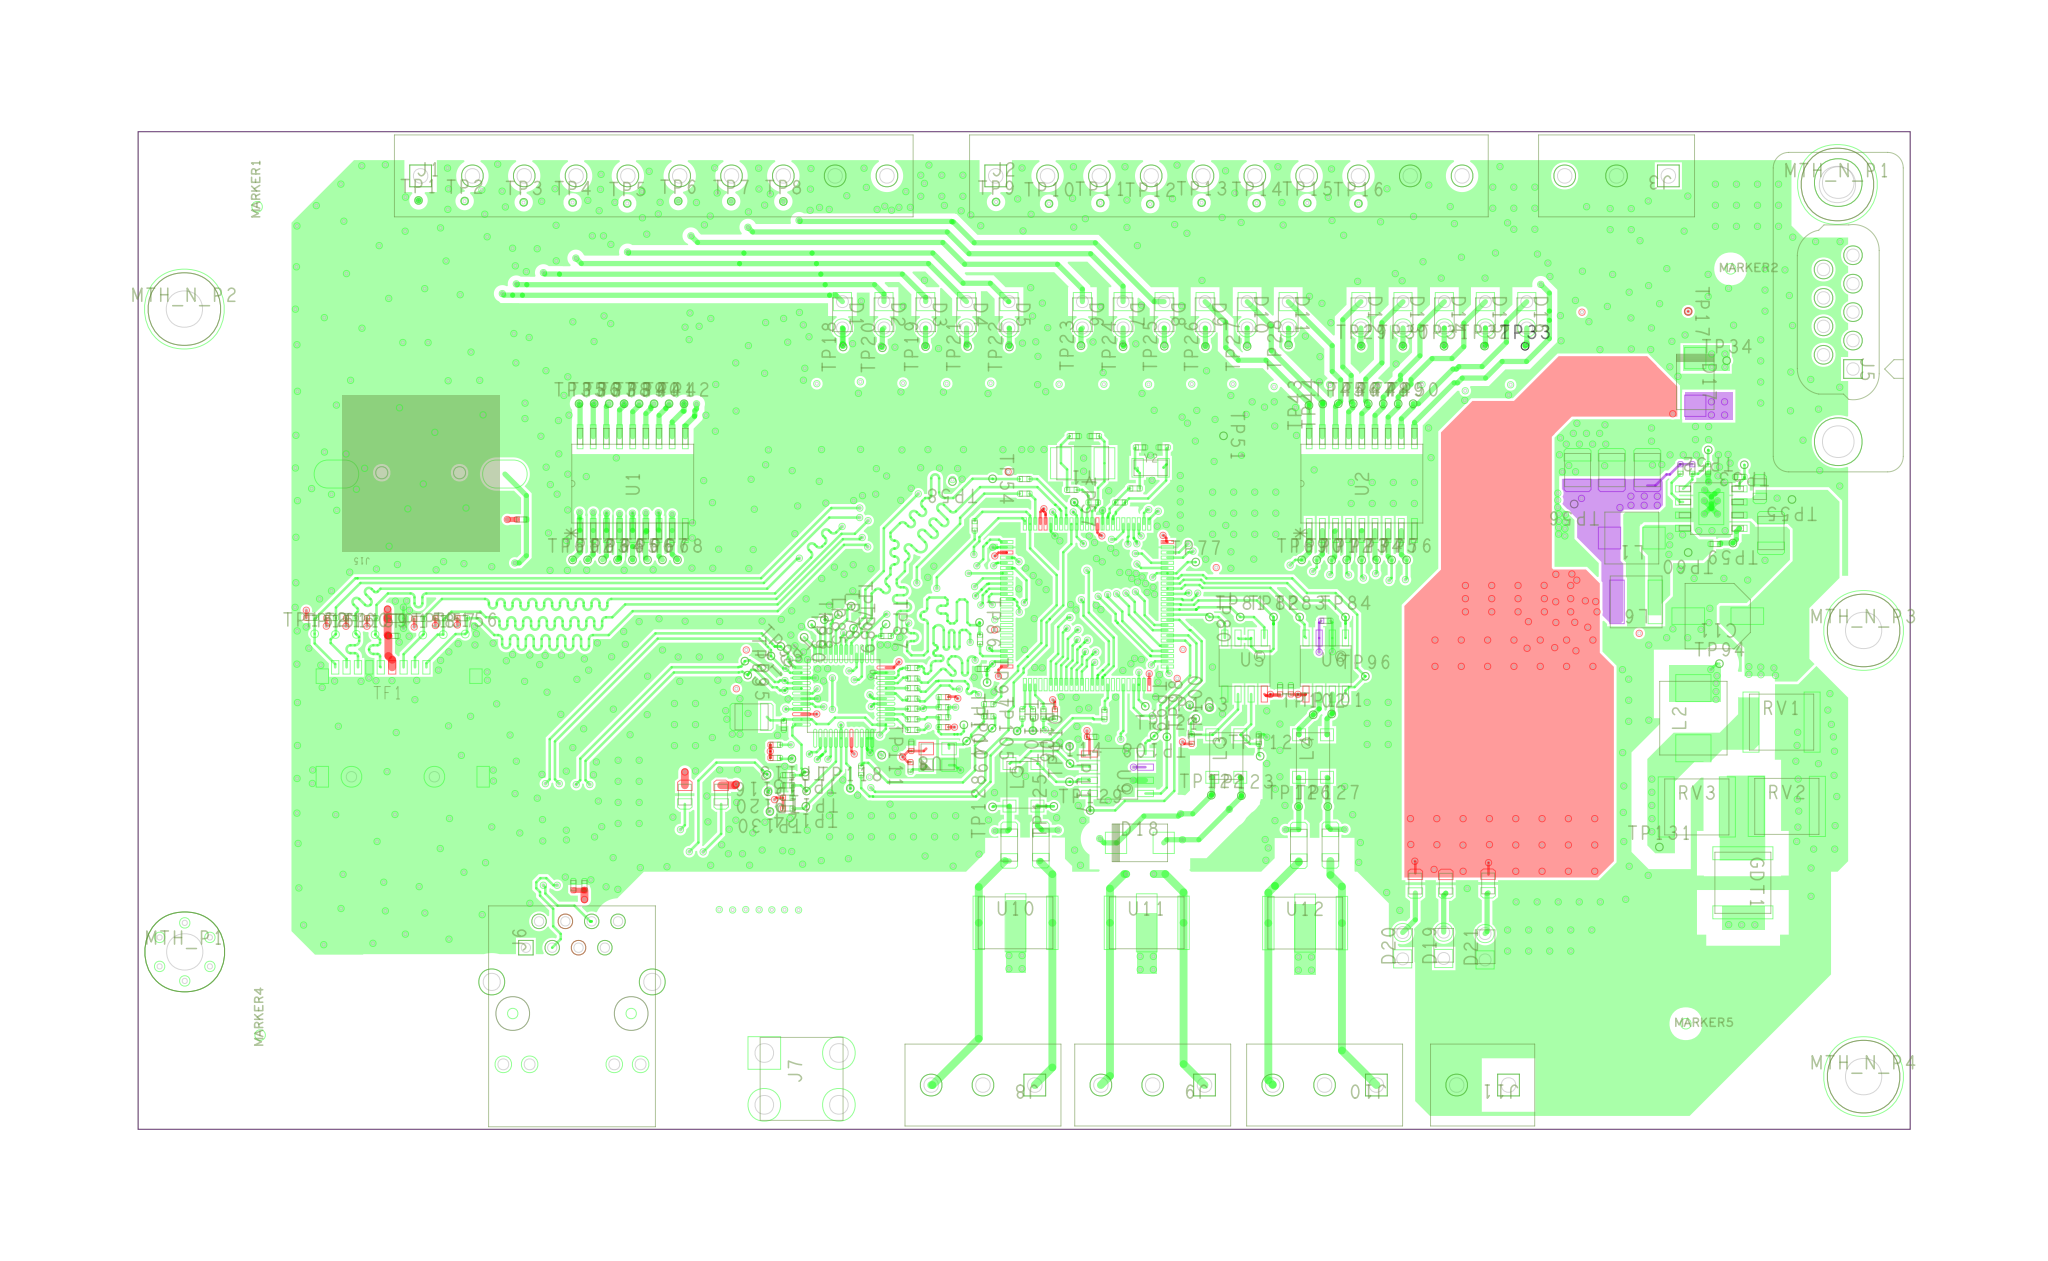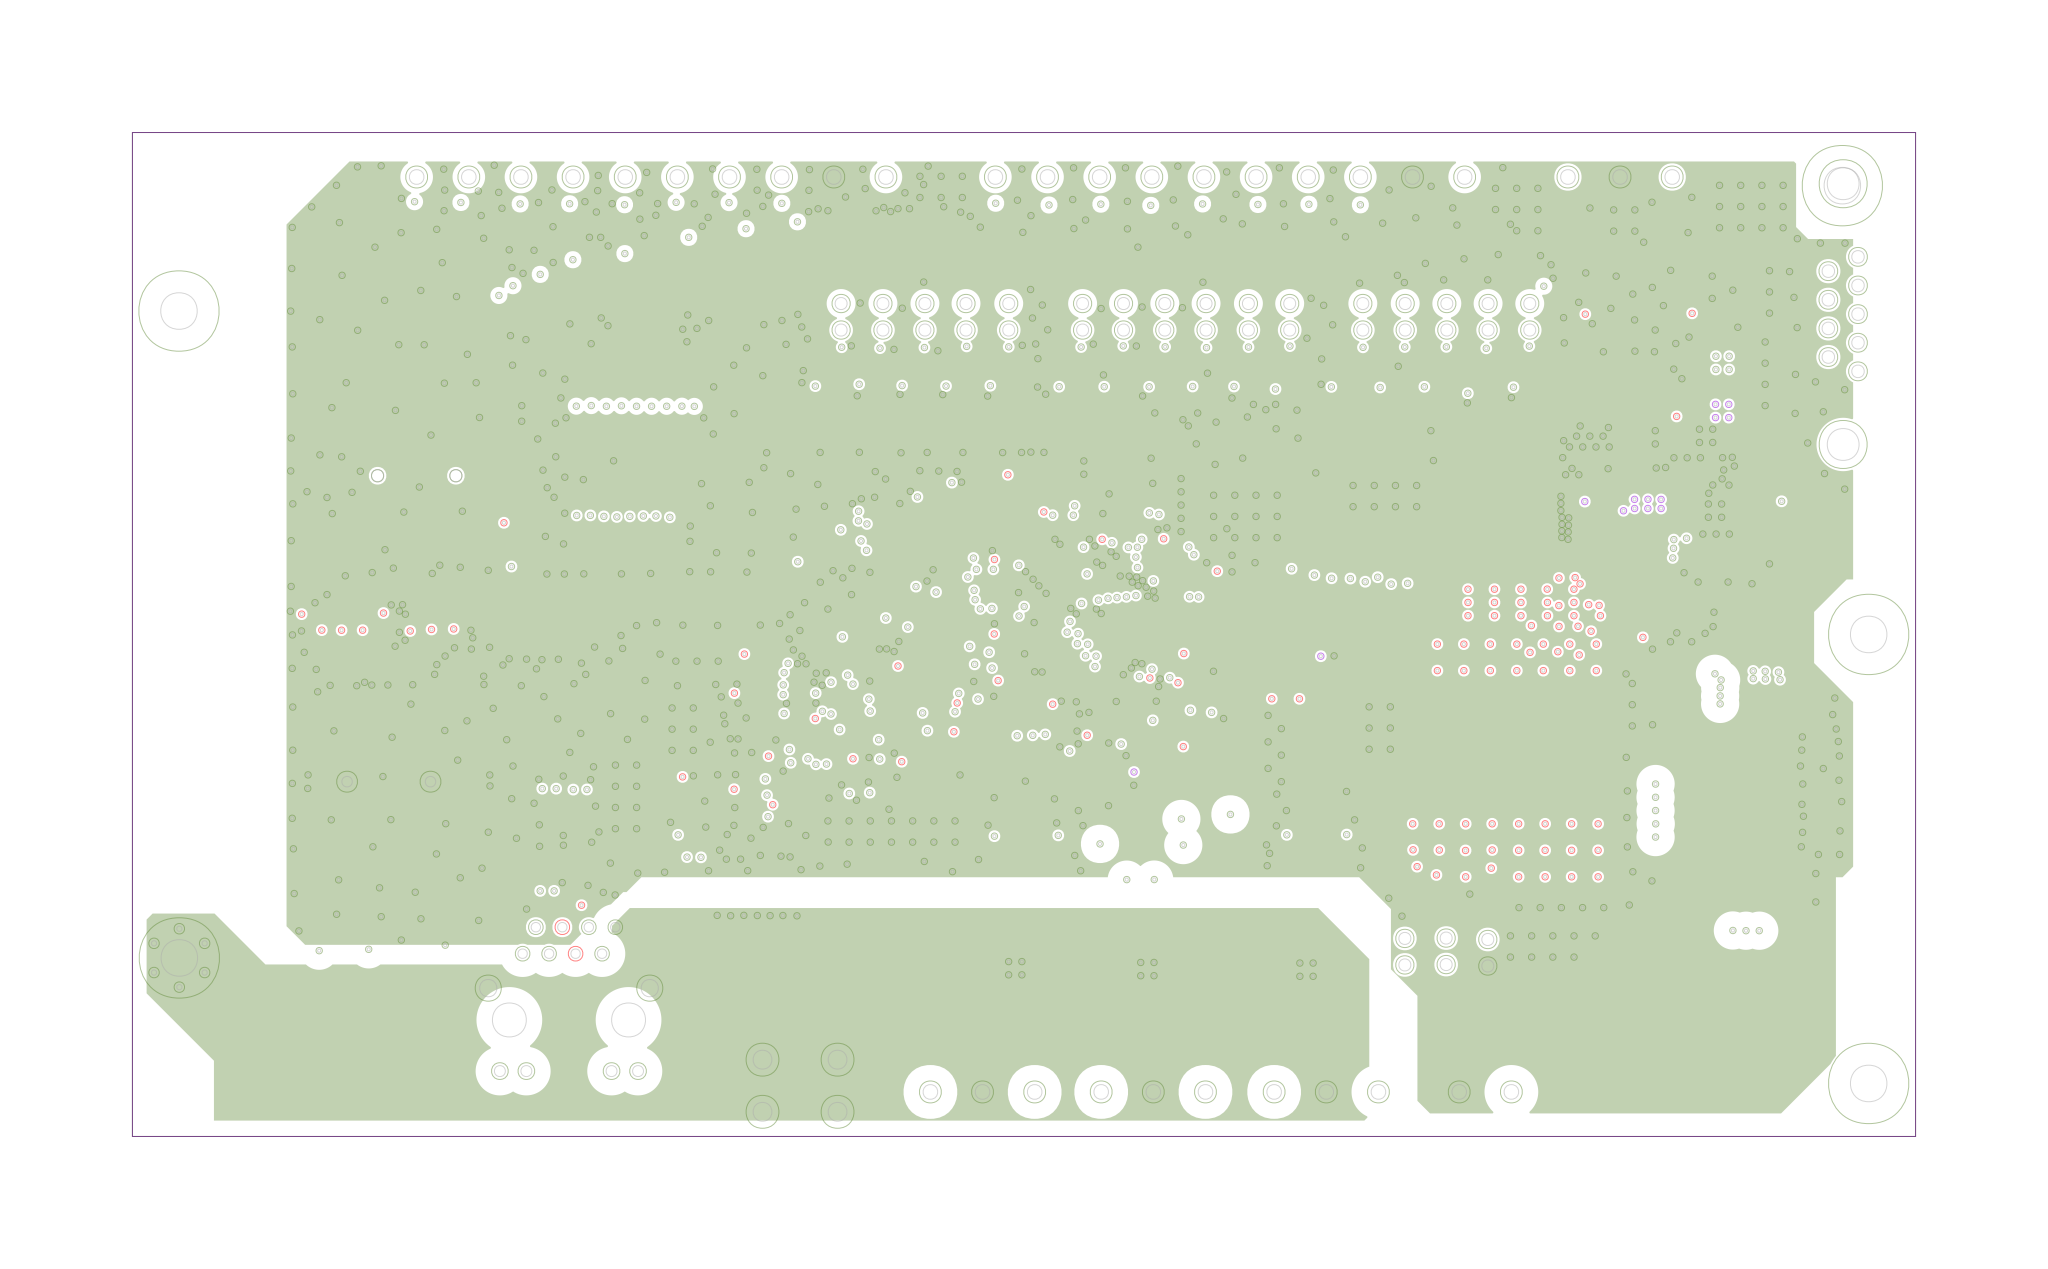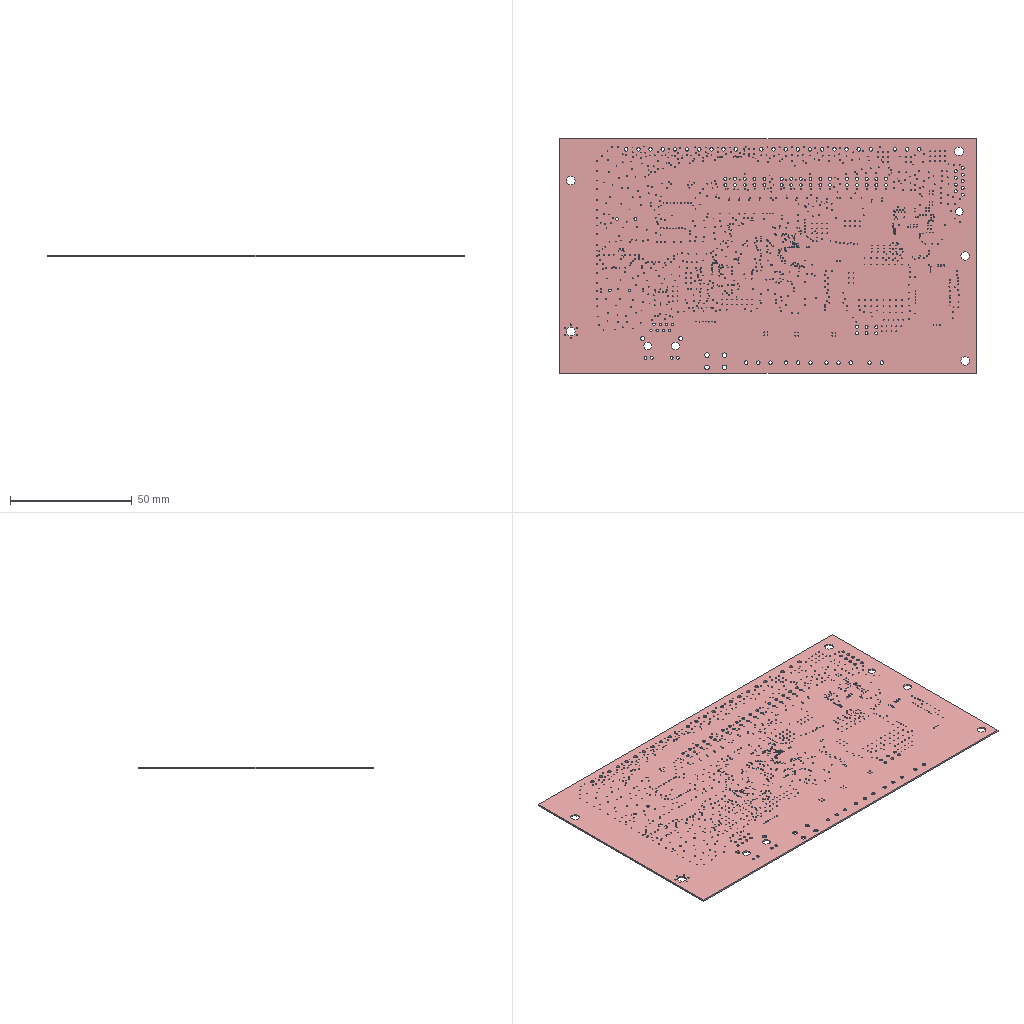Circuit board layout | Cadence Allegro | box 171 x 96.2 x 0.7 mm
Layer stack:
# Cadence Allegro layer stack of  (unit mm; from the constraint file cross-section; dielectric type: 0 not recorded (Allegro does not mark core vs prepreg), 3 surface material)
index,name,kind,layer,copper_thickness_mm,dielectric_type,dielectric_thickness_mm,dielectric_material,dielectric_constant
0,Top Surface,other,,,,,,
1,TOP,copper,TOP,0.0305,,,,
2,Dielectric1,dielectric,,,0,0.2032,FR-4,4.5
3,GND,copper,GND,0.0305,,,,
4,Dielectric2,dielectric,,,0,0.2032,FR-4,4.5
5,POWER,copper,POWER,0.0305,,,,
6,Dielectric3,dielectric,,,0,0.2032,FR-4,4.5
7,BOTTOM,copper,BOTTOM,0.0305,,,,
8,Bottom Surface,other,,,,,,
# drill layer pairs: low layer,high layer
drill_pair,TOP,BOTTOM
Part placement:
REFDES,COMP_VALUE,SYM_NAME,SYM_X,SYM_Y,SYM_ROTATE,SYM_MIRROR
C1,8PF,C0402,6855.4,7438.9,180.000,NO
C2,8PF,C0402,6931.2,7438.9,0.000,NO
C3,6PF,C0402,7106.7,7396.1,0.000,NO
C4,6PF,C0402,7192.7,7396.1,180.000,NO
C5,22uf,C1210,8767.0,7310.0,90.000,NO
C6,22uf,C1210,8897.0,7310.0,90.000,NO
C7,22uf,C1210,9032.0,7310.0,90.000,NO
C8,.22uf,C0805,9459.5,7237.7,90.000,NO
C9,4.7uf,C1210,9502.0,7071.0,270.000,NO
C10,.1uf,C0402,9290.0,7029.4,180.000,NO
C11,47uF,CAPAE630X770N,9299.6,6755.5,180.000,NO
C12,.1uf,C0402,7810.8,6737.8,180.000,NO
C13,.1uf,C0402,7637.0,6476.0,90.000,NO
C14,.1uf,C0402,7677.8,6476.0,90.000,NO
C15,10uf,C1210,5629.0,6373.0,180.000,NO
C16,.1uf,C0402,5751.5,6341.2,270.000,NO
C17,.1uf,C0402,6921.0,6297.0,0.000,NO
C18,.1uf,C0402,6236.0,6261.0,90.000,NO
C19,.1uf,C0402,5766.6,6112.8,180.000,NO
C20,.1uf,C0402,4952.1,5732.2,90.000,NO
C21,.1uf,C0402,4994.2,5731.7,90.000,NO
C22,10uf,C1210,8883.0,7307.0,0.000,YES
C23,.047uf,C0402,6454.5,7288.5,90.000,YES
C24,1uf,C0603,8901.0,7208.0,0.000,YES
C25,.1uf,C0402,6928.3,7163.6,90.000,YES
C26,.1uf,C0402,9106.6,7156.8,180.000,YES
C27,.1uf,C0402,6773.0,7207.4,270.000,YES
C28,1uf,C0603,6725.9,7224.5,270.000,YES
C29,.1uf,C0402,8652.4,7044.0,270.000,YES
C30,10uf,C1210,8564.0,7046.0,270.000,YES
C31,22uf,C1210,8415.1,7046.0,270.000,YES
C32,.1uf,C0402,7152.0,7037.0,0.000,YES
C33,.1uf,C0402,6969.6,7107.0,270.000,YES
C34,.1uf,C0402,6586.8,6986.9,270.000,YES
C35,.1uf,C0402,6867.2,7062.2,180.000,YES
C36,.047uf,C0402,6594.5,6916.1,180.000,YES
C37,.047uf,C0402,6594.8,6835.9,180.000,YES
C38,.047uf,C0402,6690.6,6722.7,180.000,YES
C39,10uf,C1210,6119.0,6632.0,270.000,YES
C40,2.2uf,C0603,6606.0,6627.0,180.000,YES
C41,.1uf,C0402,6220.5,6612.0,270.000,YES
C42,.1uf,C0402,5609.0,6587.0,90.000,YES
C43,.1uf,C0402,6607.0,6577.0,180.000,YES
C44,10uf,C1210,6662.0,6492.0,180.000,YES
C45,.1uf,C0402,7127.0,6467.0,90.000,YES
C46,.1uf,C0402,5849.0,6462.0,90.000,YES
C47,.1uf,C0402,5609.0,6462.0,90.000,YES
C48,2.2uf,C0603,7078.0,6459.0,90.000,YES
C49,.047uf,C0805,9617.0,6398.0,90.000,YES
C50,.1uf,C0402,5834.0,6357.0,0.000,YES
C51,.1uf,C0402,6129.0,6272.0,180.000,YES
C52,.1uf,C0402,6045.0,6272.0,180.000,YES
C53,.1uf,C0402,7135.0,6181.0,0.000,YES
C54,4700pf,C0603,6690.0,6178.0,0.000,YES
C55,4700pf,C0603,7790.0,6177.0,0.000,YES
C56,100PF,C0603,6568.0,5864.0,90.000,YES
C57,100PF,C0603,7878.4,5863.4,90.000,YES
C58,100PF,C0603,7656.7,5863.4,90.000,YES
C59,100PF,C0603,6781.0,5863.0,90.000,YES
C60,10nF,C1206,5675.7,5756.3,90.000,YES
C61,47nf,C1210,5549.0,5754.3,90.000,YES
C62,.1uf,C0402,4266.9,6680.5,0.000,NO
C63,2.2uf,C0603,4276.5,6747.0,0.000,NO
D1,LED,LEDRR254,5974.2,7899.6,270.000,NO
D2,LED,LEDRR254,6132.1,7899.6,270.000,NO
D3,LED,LEDRR254,6290.6,7899.6,270.000,NO
D4,LED,LEDRR254,6445.7,7899.6,270.000,NO
D5,LED,LEDRR254,6607.0,7899.6,270.000,NO
D6,LED,LEDRR254,6885.9,7899.6,270.000,NO
D7,LED,LEDRR254,7040.4,7899.6,270.000,NO
D8,LED,LEDRR254,7196.2,7899.6,270.000,NO
D9,LED,LEDRR254,7352.0,7899.6,270.000,NO
D10,LED,LEDRR254,7511.9,7899.6,270.000,NO
D11,LED,LEDRR254,7667.8,7899.6,270.000,NO
D12,LED,LEDRR254,7943.9,7899.6,270.000,NO
D13,LED,LEDRR254,8103.8,7899.6,270.000,NO
D14,LED,LEDRR254,8261.0,7899.6,270.000,NO
D15,LED,LEDRR254,8416.8,7899.6,270.000,NO
D16,LED,LEDRR254,8574.1,7899.6,270.000,NO
D17,3A,SMB,9214.2,7644.7,270.000,NO
D18,SMBJ10CA,SMB,7104.2,5894.6,0.000,NO
D19,LED,LEDRR254,8258.5,5505.6,90.000,NO
D20,LED,LEDRR254,8102.6,5504.2,90.000,NO
D21,LED,LEDRR254,8415.7,5500.2,90.000,NO
D22,BAV99,SOT-23,9196.6,8009.0,270.000,YES
D23,BAV99,SOT-23,8841.3,8009.0,270.000,YES
D24,SS26FL,SMA,9046.0,7449.0,180.000,YES
D25,SS26FL,SMA,9262.0,7013.0,180.000,YES
D26,TPSMC27CA,SMC,9187.0,6388.0,270.000,YES
D27,3A,SMB,9482.0,6353.0,90.000,YES
D28,SMBJ10CA,SMB,7504.4,6119.4,90.000,YES
D29,SMBJ10CA,SMB,7322.4,6119.4,90.000,YES
D30,UFS08A2.8L04,SOIC127P600X175-8N,4928.2,5939.4,270.000,YES
D31,SM24CANA-04HTG,SOT23,6674.0,5853.0,180.000,YES
D32,SM24CANA-04HTG,SOT23,7768.0,5852.0,180.000,YES
D33,BAV99,SOT-23,4812.0,7570.5,180.000,YES
D34,1N4148WS,SOD-323,5949.9,7724.9,180.000,YES
D35,1N4148WS,SOD-323,6117.1,7726.5,180.000,YES
D36,1N4148WS,SOD-323,6281.5,7725.8,180.000,YES
D37,1N4148WS,SOD-323,6448.9,7725.2,180.000,YES
D38,1N4148WS,SOD-323,6613.1,7725.7,180.000,YES
D39,1N4148WS,SOD-323,6873.4,7724.2,180.000,YES
D40,1N4148WS,SOD-323,7042.0,7725.1,180.000,YES
D41,1N4148WS,SOD-323,7208.3,7725.0,180.000,YES
D42,1N4148WS,SOD-323,7373.0,7725.5,180.000,YES
D43,1N4148WS,SOD-323,7536.2,7726.1,180.000,YES
D44,1N4148WS,SOD-323,7698.0,7726.5,180.000,YES
D45,1N4148WS,SOD-323,7914.2,7724.4,180.000,YES
D46,1N4148WS,SOD-323,8079.4,7724.5,180.000,YES
D47,1N4148WS,SOD-323,8247.0,7725.0,180.000,YES
D48,1N4148WS,SOD-323,8416.1,7725.3,180.000,YES
D49,1N4148WS,SOD-323,8584.0,7725.4,180.000,YES
F1,10A,FUSE10A,9312.0,6068.0,0.000,YES
GDT1,5kA,GDT5KA2P,9395.0,5743.0,270.000,NO
J1,KF127-5.0-10P,PHONEX10P500_82,4371.7,8427.0,270.000,NO
J2,KF127-5.0-10P,PHONEX10P500_82,6556.6,8427.0,270.000,NO
J3,3,PHONEX3P500,9111.9,8427.0,90.000,NO
J5,DB9,DB_V_R-9,9813.4,7693.7,270.000,NO
J6,HY911105AE,RJ_RA-8,4771.7,5496.6,0.000,NO
J7,EARTH4P,EARTH4P_M3,5819.1,4998.4,0.000,NO
J8,KF127-5.0-3P,PHONEX3P500_82,6705.0,4975.0,90.000,NO
J9,KF127-5.0-3P,PHONEX3P500_82,7349.8,4975.1,90.000,NO
J10,KF127-5.0-3P,PHONEX3P500_82,8002.8,4975.1,90.000,NO
J11,KF127-5.0-2P,PHONEX2P500_82,8504.7,4975.1,90.000,NO
J13,TS5215A 250gf,TS5215A,4858.9,7099.9,90.000,YES
J15,BAT2,CR1220,4371.9,7299.9,180.000,NO
L1,6.8uH,SPM5030,8973.0,7052.0,180.000,NO
L2,22uH,SPM6530,9207.0,6368.0,90.000,NO
L3,51uH,CM320X450X150-4N,7432.5,6224.2,0.000,NO
L4,51uH,CM320X450X150-4N,7762.0,6224.2,0.000,NO
L5,51uH,CM320X450X150-4N,6662.0,6115.0,0.000,NO
L6,6.8uH,SNR5040,8989.7,6809.5,180.000,NO
MARKER1,30mil,FIDMS0,3750.6,8309.7,90.000,NO
MARKER2,30mil,FIDMS0,9348.4,8073.9,0.000,NO
MARKER3,30mil,FIDMS0,3982.6,5332.6,0.000,YES
MARKER4,30mil,FIDMS0,3762.1,5164.7,90.000,NO
MARKER5,30mil,FIDMS0,9178.4,5207.9,0.000,NO
MARKER6,30mil,FIDMS0,3802.6,8341.2,0.000,YES
MARKER7,30mil,FIDMS0,9431.0,8157.0,0.000,YES
MARKER8,30mil,FIDMS0,9179.1,5206.0,90.000,YES
MTH_N_P1,D3.5plated,MTGP770H350P,9754.3,8394.3,0.000,NO
MTH_N_P2,D3.5plated,MTGP770H350P,3474.3,7921.3,0.000,NO
MTH_N_P3,D3.5plated,MTGP770H350P,9853.7,6701.1,0.000,NO
MTH_N_P4,D3.5plated,MTGP770H350P,9853.7,5007.0,0.000,NO
MTH_P1,D3.5plated,MTGP770H350V6P,3475.7,5480.6,0.000,NO
R1,10k,R0402,9158.0,7314.0,90.000,NO
R2,68k,R0402,9203.0,7314.0,270.000,NO
R3,12k,R0402,9263.0,7314.0,270.000,NO
R4,16.9k,R0402,9383.0,7284.0,180.000,NO
R5,33R(NC),R0402,6666.7,7276.0,180.000,NO
R6,0R,R0402,7085.6,7240.2,0.000,NO
R7,0R,R0402,6846.0,7235.0,0.000,NO
R8,0R,R0402,6666.7,7220.5,180.000,NO
R9,1M,R0402,6927.0,7187.0,180.000,NO
R10,10M,R0402,7029.2,7187.0,0.000,NO
R11,0R,R0402,6476.6,7098.2,270.000,NO
R12,33R(NC),R0402,6140.0,6680.0,180.000,NO
R13,33R,R0402,6497.0,6667.0,90.000,NO
R14,33R(NC),R0402,6240.8,6558.5,180.000,NO
R15,0R(NC),R0402,6506.0,6555.0,180.000,NO
R16,33R(NC),R0402,6240.8,6518.5,180.000,NO
R17,33R,R0402,6240.8,6482.0,180.000,NO
R18,2.2k,R0402,6358.0,6447.9,180.000,NO
R19,33R,R0402,6240.8,6442.0,180.000,NO
R20,0R,R0402,6530.0,6421.0,180.000,NO
R21,0R,R0402,6358.0,6409.5,180.000,NO
R22,33R,R0402,6240.8,6403.9,180.000,NO
R23,33R,R0402,6658.0,6384.0,270.000,NO
R24,33R,R0402,6698.0,6384.0,270.000,NO
R25,0R(NC),R0402,6738.0,6384.0,90.000,NO
R26,10k(NC),R0402,6781.5,6384.0,270.000,NO
R27,33R,R0402,6969.5,6382.0,90.000,NO
R28,0R,R0402,6530.0,6375.0,0.000,NO
R29,0R,R0402,6358.0,6371.5,180.000,NO
R30,33R,R0402,6240.8,6363.9,180.000,NO
R31,2.2k,R0402,6358.0,6334.0,180.000,NO
R32,33R(NC),R0402,6240.9,6323.5,180.000,NO
R33,10k,R0402,7301.1,6288.6,90.000,NO
R34,10k,R0402,7556.1,6288.6,270.000,NO
R35,2.2k,R0402,5719.0,6267.0,180.000,NO
R36,2.2k,R0402,5719.0,6217.0,180.000,NO
R37,10k,R0402,6233.0,6183.0,90.000,NO
R38,0R(NC),R0402,6045.5,6169.5,90.000,NO
R39,4.87k,R0402,5766.6,6151.5,180.000,NO
R40,390R,R0805,5375.6,6077.7,90.000,NO
R41,390R,R0805,5513.5,6077.7,90.000,NO
R42,10k,R0402,5766.6,6066.0,0.000,NO
R43,1.5k,R0402,5766.6,6025.0,0.000,NO
R44,4.7R,R1206,6728.0,5887.0,270.000,NO
R45,4.7R,R1206,6608.0,5886.0,270.000,NO
R46,4.7R,R1206,7828.0,5886.0,270.000,NO
R47,4.7R,R1206,7708.0,5885.0,270.000,NO
R50,390R,R0805,8150.7,5739.7,90.000,NO
R51,1k,R0805,7941.5,8236.7,270.000,YES
R52,1k,R0805,7743.5,8239.0,270.000,YES
R53,1k,R0805,7550.4,8238.3,270.000,YES
R54,1k,R0805,7348.0,8240.6,270.000,YES
R55,1k,R0805,7154.5,8235.3,270.000,YES
R56,1k,R0805,6966.3,8238.7,270.000,YES
R57,1k,R0805,6764.0,8237.0,270.000,YES
R58,1k,R0805,6560.8,8235.8,270.000,YES
R59,1k,R0805,5751.4,8233.0,270.000,YES
R60,1k,R0805,5551.3,8233.9,270.000,YES
R61,1k,R0805,5354.2,8234.7,270.000,YES
R62,1k,R0805,5157.7,8226.2,270.000,YES
R63,1k,R0805,4961.5,8230.0,270.000,YES
R64,1k,R0805,4764.0,8231.2,270.000,YES
R65,1k,R0805,4550.9,8236.6,270.000,YES
R66,1k,R0805,4379.8,8236.6,270.000,YES
R67,4.7R,R1206,9175.1,8132.4,0.000,YES
R68,4.7R,R1206,8820.7,8132.4,0.000,YES
R101,2k,R0805,7209.5,7635.4,180.000,YES
R102,2k,R0805,7040.4,7635.9,180.000,YES
R103,2k,R0805,6869.5,7635.8,180.000,YES
R104,2k,R0805,6611.2,7638.1,180.000,YES
R105,2k,R0805,6442.4,7638.2,180.000,YES
R106,2k,R0805,6276.1,7640.0,180.000,YES
R107,2k,R0805,6114.5,7640.1,180.000,YES
R108,2k,R0805,5955.9,7638.5,180.000,YES
R109,2k,R0805,8586.3,7633.9,180.000,YES
R110,2k,R0805,8414.9,7633.5,180.000,YES
R111,2k,R0805,8251.2,7633.0,180.000,YES
R112,2k,R0805,8083.2,7632.9,180.000,YES
R113,2k,R0805,7914.8,7635.1,180.000,YES
R114,2k,R0805,7697.7,7636.7,180.000,YES
R115,2k,R0805,7533.6,7636.6,180.000,YES
R116,2k,R0805,7374.3,7636.6,180.000,YES
R117,1k,R0402,9516.1,7270.6,270.000,YES
R118,10k,R0402,9478.0,7270.6,270.000,YES
R119,1k,R0402,6557.6,7265.6,0.000,YES
R120,10k,R0402,6557.6,7303.5,0.000,YES
R121,1k,R0402,6496.5,7288.6,90.000,YES
R122,10k,R0402,6889.0,7164.5,270.000,YES
R123,0R,R0402,6813.9,7126.6,90.000,YES
R124,0R(NC),R0402,6868.1,7107.7,180.000,YES
R125,10k(NC),R0402,7152.0,6977.0,0.000,YES
R126,1k,R0402,6594.9,6875.3,180.000,YES
R127,10k,R0402,7152.0,6938.9,180.000,YES
R128,33R(NC),R0402,7047.0,6953.5,0.000,YES
R129,1k,R0402,6597.2,6795.5,180.000,YES
R130,10k,R0402,7346.3,6882.9,0.000,YES
R131,10k,R0402,7346.3,6922.1,0.000,YES
R132,10k,R0402,9167.2,6876.5,270.000,YES
R135,1k,R0402,6690.4,6684.0,180.000,YES
R136,10k,R0402,9167.2,6802.5,270.000,YES
R137,10k(NC),R0402,6596.8,6716.6,180.000,YES
R138,10k,R0402,6597.0,6756.7,0.000,YES
R139,49.9R,R0603,5689.0,6632.0,0.000,YES
R140,0R,R0402,7362.0,6623.0,180.000,YES
R141,10k,R0402,7223.0,6621.2,0.000,YES
R142,10k,R0402,7362.0,6586.0,180.000,YES
R143,0R,R0402,7223.0,6584.0,180.000,YES
R144,49.9R,R0603,5689.0,6572.0,0.000,YES
R145,49.9R,R0603,5689.0,6507.0,0.000,YES
R146,10k,R0402,7223.0,6496.2,0.000,YES
R147,0R,R0402,7223.0,6459.0,180.000,YES
R148,49.9R,R0603,5689.0,6447.0,0.000,YES
R149,33R(NC),R0402,6181.5,6440.5,0.000,YES
R150,33R(NC),R0402,6181.5,6396.5,0.000,YES
R151,10k,R0402,6916.1,6152.6,270.000,YES
R152,1k,R0402,6867.0,6152.6,270.000,YES
R153,2.2k,R0402,5629.0,6146.0,0.000,YES
R154,2.2k,R0402,5629.0,6076.0,0.000,YES
R155,62R,R1206,6719.0,6043.0,270.000,YES
R156,62R,R1206,6622.0,6043.0,270.000,YES
R157,62R,R1206,7819.0,6042.0,270.000,YES
R158,62R,R1206,7722.0,6042.0,270.000,YES
R159,2.2k,R0402,5629.0,6016.0,0.000,YES
R160,62R,R1206,7476.7,5829.0,90.000,YES
R161,62R,R1206,7359.3,5829.0,90.000,YES
R162,4.7R,R1206,7222.3,5829.0,90.000,YES
R163,4.7R,R1206,6993.3,5823.9,90.000,YES
R164,1M,R1206,5771.4,5756.3,90.000,YES
R165,4.7R,R1206,4828.4,7432.3,0.000,YES
R166,2k,R0805,8427.3,5740.4,270.000,NO
R167,2k,R0805,8266.4,5739.4,270.000,NO
R200,10k,R0402,4529.7,6747.5,0.000,NO
R201,10k,R0402,4446.0,6747.5,0.000,NO
R202,10k,R0402,4365.6,6745.3,0.000,NO
R203,10k,R0402,4185.9,6747.5,0.000,NO
R204,10k,R0402,4106.4,6747.6,0.000,NO
R205,10k,R0402,4031.8,6748.2,0.000,NO
R206,10k,R0402,3955.8,6749.0,0.000,NO
R207,0R(NC),R0402,4755.3,7122.4,180.000,NO
RT1,10K,R0603,9114.2,6851.8,270.000,YES
RV1,47V,R2220,9542.0,6353.0,0.000,NO
RV2,47V,R2220,9562.0,6033.0,0.000,NO
RV3,47V,R2220,9220.0,6031.0,0.000,NO
TF1,TF-01A,TF-01A,3998.4,6145.6,0.000,NO
TP1,TP,TPAD_30MIL,4363.8,8333.8,0.000,NO
TP2,TP,TPAD_30MIL,4539.1,8331.5,0.000,NO
TP3,TP,TPAD_30MIL,4763.4,8326.7,0.000,NO
TP4,TP,TPAD_30MIL,4949.2,8326.0,0.000,NO
TP5,TP,TPAD_30MIL,5156.6,8322.4,0.000,NO
TP6,TP,TPAD_30MIL,5350.5,8331.3,0.000,NO
TP7,TP,TPAD_30MIL,5551.7,8330.3,0.000,NO
TP8,TP,TPAD_30MIL,5749.7,8330.0,0.000,NO
TP9,TP,TPAD_30MIL,6557.8,8328.0,0.000,NO
TP10,TP,TPAD_30MIL,6759.0,8321.4,0.000,NO
TP11,TP,TPAD_30MIL,6954.0,8323.9,0.000,NO
TP12,TP,TPAD_30MIL,7143.7,8320.0,0.000,NO
TP13,TP,TPAD_30MIL,7338.9,8325.3,0.000,NO
TP14,TP,TPAD_30MIL,7547.8,8323.3,0.000,NO
TP15,TP,TPAD_30MIL,7740.2,8324.2,0.000,NO
TP16,TP,TPAD_30MIL,7934.6,8322.0,0.000,NO
TP17,TP,TPAD_30MIL,9187.3,7912.2,270.000,NO
TP18,TP,TPAD_30MIL,5976.8,7777.5,90.000,NO
TP19,TP,TPAD_30MIL,6290.0,7778.8,90.000,NO
TP20,TP,TPAD_30MIL,6125.8,7774.4,90.000,NO
TP21,TP,TPAD_30MIL,6450.0,7779.4,90.000,NO
TP22,TP,TPAD_30MIL,6608.6,7777.5,90.000,NO
TP23,TP,TPAD_30MIL,6880.5,7782.1,90.000,NO
TP24,TP,TPAD_30MIL,7040.5,7778.4,90.000,NO
TP25,TP,TPAD_30MIL,7197.1,7780.0,90.000,NO
TP26,TP,TPAD_30MIL,7353.3,7779.0,90.000,NO
TP27,TP,TPAD_30MIL,7511.7,7779.4,90.000,NO
TP28,TP,TPAD_30MIL,7669.2,7784.7,90.000,NO
TP29,TP,TPAD_30MIL,7945.0,7780.5,0.000,NO
TP30,TP,TPAD_30MIL,8103.4,7780.2,0.000,NO
TP31,TP,TPAD_30MIL,8259.8,7780.1,0.000,NO
TP32,TP,TPAD_30MIL,8413.9,7780.7,0.000,NO
TP33,TP,TPAD_30MIL,8567.5,7780.1,0.000,NO
TP34,TP,TPAD_30MIL,9333.6,7725.6,0.000,NO
TP35,TP,TPAD_30MIL,4973.5,7562.0,0.000,NO
TP36,TP,TPAD_30MIL,5031.0,7562.0,0.000,NO
TP37,TP,TPAD_30MIL,5088.0,7562.0,0.000,NO
TP38,TP,TPAD_30MIL,5144.8,7562.0,0.000,NO
TP39,TP,TPAD_30MIL,5201.8,7562.0,0.000,NO
TP40,TP,TPAD_30MIL,5258.6,7562.0,0.000,NO
TP41,TP,TPAD_30MIL,5315.6,7562.0,0.000,NO
TP42,TP,TPAD_30MIL,5372.4,7562.0,0.000,NO
TP43,TP,TPAD_30MIL,7746.6,7555.7,90.000,NO
TP44,TP,TPAD_30MIL,7798.9,7560.9,90.000,NO
TP45,TP,TPAD_30MIL,7858.0,7562.0,0.000,NO
TP46,TP,TPAD_30MIL,7914.8,7562.0,0.000,NO
TP47,TP,TPAD_30MIL,7971.8,7562.0,0.000,NO
TP48,TP,TPAD_30MIL,8028.6,7562.0,0.000,NO
TP49,TP,TPAD_30MIL,8085.6,7562.0,0.000,NO
TP50,TP,TPAD_30MIL,8142.4,7562.0,0.000,NO
TP51,TP,TPAD_30MIL,7422.0,7440.0,270.000,NO
TP52,TP,TPAD_30MIL,9263.6,7386.4,180.000,NO
TP53,TP,TPAD_30MIL,9400.4,7330.2,180.000,NO
TP54,TP,TPAD_30MIL,6544.6,7276.9,270.000,NO
TP55,TP,TPAD_30MIL,9581.6,7198.4,180.000,NO
TP56,TP,TPAD_30MIL,8754.2,7181.1,180.000,NO
TP57,TP,TPAD_30MIL,6854.8,7188.4,270.000,NO
TP58,TP,TPAD_30MIL,6392.2,7266.4,180.000,NO
TP59,TP,TPAD_30MIL,9357.2,7033.0,180.000,NO
TP60,TP,TPAD_30MIL,9187.2,6997.0,180.000,NO
TP61,TP,TPAD_30MIL,4949.2,6969.0,0.000,NO
TP62,TP,TPAD_30MIL,5006.2,6969.0,0.000,NO
TP63,TP,TPAD_30MIL,5063.0,6969.0,0.000,NO
TP64,TP,TPAD_30MIL,5120.0,6969.0,0.000,NO
TP65,TP,TPAD_30MIL,5176.8,6969.0,0.000,NO
TP66,TP,TPAD_30MIL,5233.8,6969.0,0.000,NO
TP67,TP,TPAD_30MIL,5290.6,6969.0,0.000,NO
TP68,TP,TPAD_30MIL,5347.6,6969.0,0.000,NO
TP69,TP,TPAD_30MIL,7719.2,6969.0,0.000,NO
TP70,TP,TPAD_30MIL,7776.2,6969.0,0.000,NO
TP71,TP,TPAD_30MIL,7833.0,6969.0,0.000,NO
TP72,TP,TPAD_30MIL,7890.0,6969.0,0.000,NO
TP73,TP,TPAD_30MIL,7946.8,6969.0,0.000,NO
TP74,TP,TPAD_30MIL,8003.8,6969.0,0.000,NO
TP75,TP,TPAD_30MIL,8060.6,6969.0,0.000,NO
TP76,TP,TPAD_30MIL,8117.6,6969.0,0.000,NO
TP77,TP,TPAD_30MIL,7316.4,6960.8,0.000,NO
TP78,TP,TPAD_30MIL,5958.8,6761.4,270.000,NO
TP79,TP,TPAD_30MIL,6007.4,6793.5,270.000,NO
TP80,TP,TPAD_30MIL,7368.6,6752.0,270.000,NO
TP81,TP,TPAD_30MIL,7485.6,6752.0,0.000,NO
TP82,TP,TPAD_30MIL,7612.0,6752.0,0.000,NO
TP83,TP,TPAD_30MIL,7711.2,6752.0,0.000,NO
TP84,TP,TPAD_30MIL,7885.4,6752.0,0.000,NO
TP85,TP,TPAD_30MIL,5905.5,6742.2,270.000,NO
TP86,TP,TPAD_30MIL,6495.0,6731.2,270.000,NO
TP87,TP,TPAD_30MIL,6140.0,6725.2,270.000,NO
TP88,TP,TPAD_30MIL,5857.3,6724.6,270.000,NO
TP89,TP,TPAD_30MIL,6016.6,6709.4,270.000,NO
TP90,TP,TPAD_30MIL,5828.8,6675.2,270.000,NO
TP91,TP,TPAD_30MIL,5740.0,6640.2,225.000,NO
TP92,TP,TPAD_30MIL,5702.6,6604.0,315.000,NO
TP93,TP,TPAD_30MIL,5603.6,6584.6,270.000,NO
TP94,TP,TPAD_30MIL,9305.8,6575.0,0.000,NO
TP95,TP,TPAD_30MIL,5614.6,6531.4,270.000,NO
TP96,TP,TPAD_30MIL,7960.8,6527.0,0.000,NO
TP97,TP,TPAD_30MIL,6523.8,6503.4,270.000,NO
TP98,TP,TPAD_30MIL,7293.2,6418.4,90.000,NO
TP99,TP,TPAD_30MIL,7124.8,6413.2,270.000,NO
TP100,TP,TPAD_30MIL,7368.2,6408.6,90.000,NO
TP101,TP,TPAD_30MIL,7833.0,6384.0,0.000,NO
TP102,TP,TPAD_30MIL,7762.6,6381.0,0.000,NO
TP103,TP,TPAD_30MIL,7316.4,6366.6,0.000,NO
TP104,TP,TPAD_30MIL,6435.6,6342.8,270.000,NO
TP105,TP,TPAD_30MIL,6542.8,6329.8,270.000,NO
TP106,TP,TPAD_30MIL,6697.8,6320.6,270.000,NO
TP107,TP,TPAD_30MIL,6637.8,6319.2,270.000,NO
TP108,TP,TPAD_30MIL,7158.4,6300.2,180.000,NO
TP109,TP,TPAD_30MIL,6445.8,6281.0,270.000,NO
TP110,TP,TPAD_30MIL,6837.2,6261.0,90.000,NO
TP111,TP,TPAD_30MIL,6123.6,6227.4,270.000,NO
TP112,TP,TPAD_30MIL,7561.2,6223.6,0.000,NO
TP113,TP,TPAD_30MIL,5782.4,6213.4,180.000,NO
TP114,TP,TPAD_30MIL,6838.8,6195.6,0.000,NO
TP115,TP,TPAD_30MIL,5832.6,6163.2,180.000,NO
TP116,TP,TPAD_30MIL,5688.0,6153.4,180.000,NO
TP117,TP,TPAD_30MIL,6836.6,6126.4,270.000,NO
TP118,TP,TPAD_30MIL,6004.0,6101.6,0.000,NO
TP119,TP,TPAD_30MIL,5838.0,6091.2,180.000,NO
TP120,TP,TPAD_30MIL,5691.8,6088.4,180.000,NO
TP121,TP,TPAD_30MIL,7207.0,6297.2,0.000,NO
TP122,TP,TPAD_30MIL,7375.6,6075.6,0.000,NO
TP123,TP,TPAD_30MIL,7489.8,6073.6,0.000,NO
TP124,TP,TPAD_30MIL,5835.2,6033.4,180.000,NO
TP125,TP,TPAD_30MIL,6777.4,6033.2,90.000,NO
TP126,TP,TPAD_30MIL,7707.0,6032.6,0.000,NO
TP127,TP,TPAD_30MIL,7818.2,6032.6,0.000,NO
TP128,TP,TPAD_30MIL,6544.6,6031.2,90.000,NO
TP129,TP,TPAD_30MIL,6915.8,6017.8,0.000,NO
TP130,TP,TPAD_30MIL,5698.8,6013.6,180.000,NO
TP131,TP,TPAD_30MIL,9077.8,5878.8,0.000,NO
TP156,TP,TPAD_30MIL,4541.4,6687.4,0.000,NO
TP157,TP,TPAD_30MIL,4457.8,6685.3,0.000,NO
TP158,TP,TPAD_30MIL,4380.0,6683.7,0.000,NO
TP159,TP,TPAD_30MIL,4198.7,6685.3,0.000,NO
TP160,TP,TPAD_30MIL,4128.0,6686.3,0.000,NO
TP161,TP,TPAD_30MIL,4048.3,6685.7,0.000,NO
TP162,TP,TPAD_30MIL,3969.2,6688.4,0.000,NO
U1,ULN2803ADWR,DW18,5177.5,7258.5,90.000,NO
U2,ULN2803ADWR,DW18,7947.5,7258.5,90.000,NO
U3,LMR16010PDDAR,DDA0008E_N,9275.2,7163.8,180.000,NO
U4,STM32F407VET6,LQFP100-14X14MM,6903.6,6800.4,270.000,NO
U5,MAX3485EESA,SOIC127P600X175-8N,7502.0,6566.0,270.000,NO
U6,TJA1044GT/3Z,SOIC127P600X175-8N,7810.3,6566.0,270.000,NO
U7,DP83848IVVX/NOPB,VBH48A_N,5979.0,6452.0,270.000,NO
U8,ECS-3225MV-500-CN-TR,OSCSC210P250X320X110-4N,6336.0,6221.0,90.000,NO
U9,TJA1044GT/3Z,SOIC127P600X175-8N,7019.0,6157.0,180.000,NO
U10,5kA,GDT3P,6632.0,5591.0,0.000,NO
U11,5kA,GDT3P,7130.4,5591.0,0.000,NO
U12,5kA,GDT3P,7732.0,5590.0,0.000,NO
U13,AMS1117-3.3,SOT223,8845.0,6988.0,90.000,YES
Y1,NX5032GA-25.000M,XTAL500X320X150N,6887.0,7336.0,180.000,NO
Y2,XDMCZLNDDF-32.768K,XTAL320X150X90N,7144.9,7318.6,0.000,NO
Pad and via stacks:
# Allegro (Cadence) via spans and padstacks; design units: ("mils" 1 10)
# via spans: padstack,start_layer,end_layer,net_example,count
VIA024D012,ETCH/TOP,ETCH/BOTTOM,GND,1233
# Allegro padstack definitions: name,start_layer,end_layer,drill,plating,holeType,type
PCM40S120,"ETCH/TOP","ETCH/TOP",0.0,"PLATED","none","smd"
TPAD_30MIL,"ETCH/TOP","ETCH/TOP",0.0,"PLATED","none","smd"
S205,"ETCH/TOP","ETCH/TOP",0.0,"PLATED","none","smd"
R580_125,"ETCH/TOP","ETCH/TOP",0.0,"PLATED","none","smd"
C770H350,"ETCH/TOP","ETCH/BOTTOM",137.8,"PLATED","circle_drill","through"
R580_155,"ETCH/TOP","ETCH/TOP",0.0,"PLATED","none","smd"
R295_200,"ETCH/TOP","ETCH/TOP",0.0,"PLATED","none","smd"
R315_220,"ETCH/TOP","ETCH/TOP",0.0,"PLATED","none","smd"
R2XR3P5,"ETCH/TOP","ETCH/TOP",0.0,"PLATED","none","smd"
R340_260,"ETCH/TOP","ETCH/TOP",0.0,"PLATED","none","smd"
R100_70,"ETCH/TOP","ETCH/TOP",0.0,"PLATED","none","smd"
R240_155,"ETCH/TOP","ETCH/TOP",0.0,"PLATED","none","smd"
SQ2,"ETCH/TOP","ETCH/TOP",0.0,"PLATED","none","smd"
S210H140T190_225_50,"ETCH/TOP","ETCH/BOTTOM",55.1,"PLATED","circle_drill","through"
C210H140T190_225_50,"ETCH/TOP","ETCH/BOTTOM",55.1,"PLATED","circle_drill","through"
C150,"ETCH/TOP","ETCH/TOP",0.0,"PLATED","none","smd"
R10240570000200A,"ETCH/TOP","ETCH/TOP",0.0,"PLATED","none","smd"
R10941220000200A,"ETCH/TOP","ETCH/TOP",0.0,"PLATED","none","smd"
R215_210,"ETCH/TOP","ETCH/TOP",0.0,"PLATED","none","smd"
R315_160,"ETCH/TOP","ETCH/TOP",0.0,"PLATED","none","smd"
R215_95,"ETCH/TOP","ETCH/TOP",0.0,"PLATED","none","smd"
R325_215,"ETCH/TOP","ETCH/TOP",0.0,"PLATED","none","smd"
R125_115,"ETCH/TOP","ETCH/TOP",0.0,"PLATED","none","smd"
R515_110,"ETCH/TOP","ETCH/TOP",0.0,"PLATED","none","smd"
SMD56X20,"ETCH/TOP","ETCH/TOP",0.0,"PLATED","none","smd"
R155_60,"ETCH/TOP","ETCH/TOP",0.0,"PLATED","none","smd"
SOT23PAD,"ETCH/TOP","ETCH/TOP",0.0,"PLATED","none","smd"
RX47Y12D0T,"ETCH/TOP","ETCH/TOP",0.0,"PLATED","none","smd"
R215_130,"ETCH/TOP","ETCH/TOP",0.0,"PLATED","none","smd"
R1P1X1P8,"ETCH/TOP","ETCH/TOP",0.0,"PLATED","none","smd"
R300_200,"ETCH/TOP","ETCH/TOP",0.0,"PLATED","none","smd"
O1011810689000000P,"ETCH/TOP","ETCH/TOP",0.0,"PLATED","none","smd"
R120_110,"ETCH/TOP","ETCH/TOP",0.0,"PLATED","none","smd"
R1P2X1P4,"ETCH/TOP","ETCH/TOP",0.0,"PLATED","none","smd"
VIA024D012,"ETCH/TOP","ETCH/BOTTOM",12.0,"PLATED","circle_drill","through"
C0402,"ETCH/TOP","ETCH/TOP",0.0,"NON_PLATED","none","smd"
C1210,"ETCH/TOP","ETCH/TOP",0.0,"NON_PLATED","none","smd"
C0603,"ETCH/TOP","ETCH/TOP",0.0,"NON_PLATED","none","smd"
C0805,"ETCH/TOP","ETCH/TOP",0.0,"NON_PLATED","none","smd"
C1206,"ETCH/TOP","ETCH/TOP",0.0,"NON_PLATED","none","smd"
C175H115T165_200_40,"ETCH/TOP","ETCH/BOTTOM",45.3,"PLATED","circle_drill","through"
S175H115T165_200_40,"ETCH/TOP","ETCH/BOTTOM",45.3,"PLATED","circle_drill","through"
PTH_C1P1C1P4,"ETCH/TOP","ETCH/BOTTOM",43.3,"PLATED","circle_drill","through"
PTH_C1P1SQ1P4,"ETCH/TOP","ETCH/BOTTOM",43.3,"PLATED","circle_drill","through"
C460H305T355_410_50,"ETCH/TOP","ETCH/BOTTOM",120.1,"PLATED","circle_drill","through"
C180H120T170_205_45,"ETCH/TOP","ETCH/BOTTOM",47.2,"PLATED","circle_drill","through"
S180H120T170_205_45,"ETCH/TOP","ETCH/BOTTOM",47.2,"PLATED","circle_drill","through"
C160H105T155_190_40,"ETCH/TOP","ETCH/BOTTOM",41.3,"PLATED","circle_drill","through"
C100HN325,"ETCH/TOP","ETCH/BOTTOM",128.0,"NON_PLATED","circle_drill","through"
C250H165T215_255_45,"ETCH/TOP","ETCH/BOTTOM",65.0,"PLATED","circle_drill","through"
C140H90T140_170_40,"ETCH/TOP","ETCH/BOTTOM",35.4,"PLATED","circle_drill","through"
S140H90T140_170_40,"ETCH/TOP","ETCH/BOTTOM",35.4,"PLATED","circle_drill","through"
V100H50,"ETCH/TOP","ETCH/BOTTOM",19.7,"PLATED","circle_drill","through"
R0402,"ETCH/TOP","ETCH/TOP",0.0,"NON_PLATED","none","smd"
R0805,"ETCH/TOP","ETCH/TOP",0.0,"NON_PLATED","none","smd"
R1206,"ETCH/TOP","ETCH/TOP",0.0,"NON_PLATED","none","smd"
SMD12X20,"ETCH/TOP","ETCH/TOP",0.0,"PLATED","none","smd"
SMD12X14,"ETCH/TOP","ETCH/TOP",0.0,"PLATED","none","smd"
THRUD1,"ETCH/TOP","ETCH/BOTTOM",39.4,"PLATED","circle_drill","through"
SMD07X13,"ETCH/TOP","ETCH/TOP",0.0,"PLATED","none","smd"
RX91Y22D0T,"ETCH/TOP","ETCH/TOP",0.0,"NON_PLATED","none","smd"
C315H210T260_305_45,"ETCH/TOP","ETCH/BOTTOM",82.7,"PLATED","circle_drill","through"
S315H210T260_305_45,"ETCH/TOP","ETCH/BOTTOM",82.7,"PLATED","circle_drill","through"
R1P0X1P9,"ETCH/TOP","ETCH/TOP",0.0,"PLATED","none","smd"
R1P4X4P2,"ETCH/TOP","ETCH/TOP",0.0,"PLATED","none","smd"
SMD4R3X2R7MMOB,"ETCH/TOP","ETCH/TOP",0.0,"NON_PLATED","none","smd"
NPAD46,"ETCH/TOP","ETCH/BOTTOM",46.0,"NON_PLATED","circle_drill","through"
VIA032D014,"ETCH/TOP","ETCH/BOTTOM",14.0,"PLATED","circle_drill","through"
C315H180T260_305_45,"ETCH/TOP","ETCH/BOTTOM",70.9,"PLATED","circle_drill","through"
S315H180T260_305_45,"ETCH/TOP","ETCH/BOTTOM",70.9,"PLATED","circle_drill","through"
R1P1X2P0,"ETCH/TOP","ETCH/TOP",0.0,"PLATED","none","smd"
R90_50,"ETCH/TOP","ETCH/TOP",0.0,"PLATED","none","smd"
Design rules, without the lines most boards share, first 10 of 36 lines:
# Cadence Allegro design rules of  (from the Constraint Manager export constraints.dcfx, design unit mil; typed fields in mm)
# columns: name | kind | enabled | priority | scope1 | scope2 | descriptor | typed fields (field=value)
# Allegro precedence (priority 1 wins): 1 Region class-to-class, 2 Region class, 3 Region, 4 class-to-class, 5 DiffPair/Bus/NetGroup override, 6 NetClass, 7 constraint set (CSet) default
# per-layer values are written LAYER=value in the descriptor and LAYER:mm in the typed field; a maximum of 0 means no limit set
# --- net classes (and buses / net groups) ---
HV | NetClass | enabled | 6 | N00275, N00563, POWER_IN, N02752 | All | Net Class (members: 4 Net) |
HV_PH | NetClass | enabled | 6 | N00275, N00563, POWER_IN, N02752 | All | Net Class (members: 4 Net) |
# --- track widths, neck and differential-pair gap (physical constraint sets) ---
SIGNAL | PhysicalCSet | enabled | 7 | not referenced | All | Physical Constraint (Min Line Width=10mil) (Max Line Width=0mil) (Min Neck Width=10mil) (Max Neck Length=0mil) (DiffPair Primary Gap=0mil) (DiffPair Neck Gap=0mil) (DiffPair Min Space=10mil) (DiffPair Coupled +Tol=0mil) (DiffPair Coupled -Tol=0mil) (Min BB Via Stagger=10mil) (Max BB Via Stagger=0mil) (T-junctions=ANYWHERE) (Pad-pad direct connect=ALL_ALLOWED) (Allowed vias=VIA024D012, VIA032D014) | min_line_width=0.254 min_neck_width=0.254 min_bvia_stagger=0.254 max_bvia_stagger=0 ts_allowed=ANYWHERE diffp_primary_gap=0 diffp_neck_gap=0 max_line_width=0 maximum_neck_length=0 pad_pad_direct_connect=ALL_ALLOWED allow_on_etch_subclass=TRUE diffp_coupled_plus=0 diffp_coupled_minus=0 diffp_min_space=0.254 vias=VIA024D012,VIA032D014
POWER | PhysicalCSet | enabled | 7 | not referenced | All | Physical Constraint (Min Line Width=30mil) (Max Line Width=0mil) (Min Neck Width=30mil) (Max Neck Length=0mil) (DiffPair Primary Gap=0mil) (DiffPair Neck Gap=0mil) (DiffPair Min Space=12mil) (DiffPair Coupled +Tol=0mil) (DiffPair Coupled -Tol=0mil) (Min BB Via Stagger=12mil) (Max BB Via Stagger=0mil) (T-junctions=ANYWHERE) (Pad-pad direct connect=ALL_ALLOWED) (Allowed vias=VIA024D012, VIA032D014) | min_line_width=0.762 min_neck_width=0.762 min_bvia_stagger=0.3048 max_bvia_stagger=0 ts_allowed=ANYWHERE diffp_primary_gap=0 diffp_neck_gap=0 max_line_width=0 maximum_neck_length=0 pad_pad_direct_connect=ALL_ALLOWED allow_on_etch_subclass=TRUE diffp_coupled_plus=0 diffp_coupled_minus=0 diffp_min_space=0.3048 vias=VIA024D012,VIA032D014